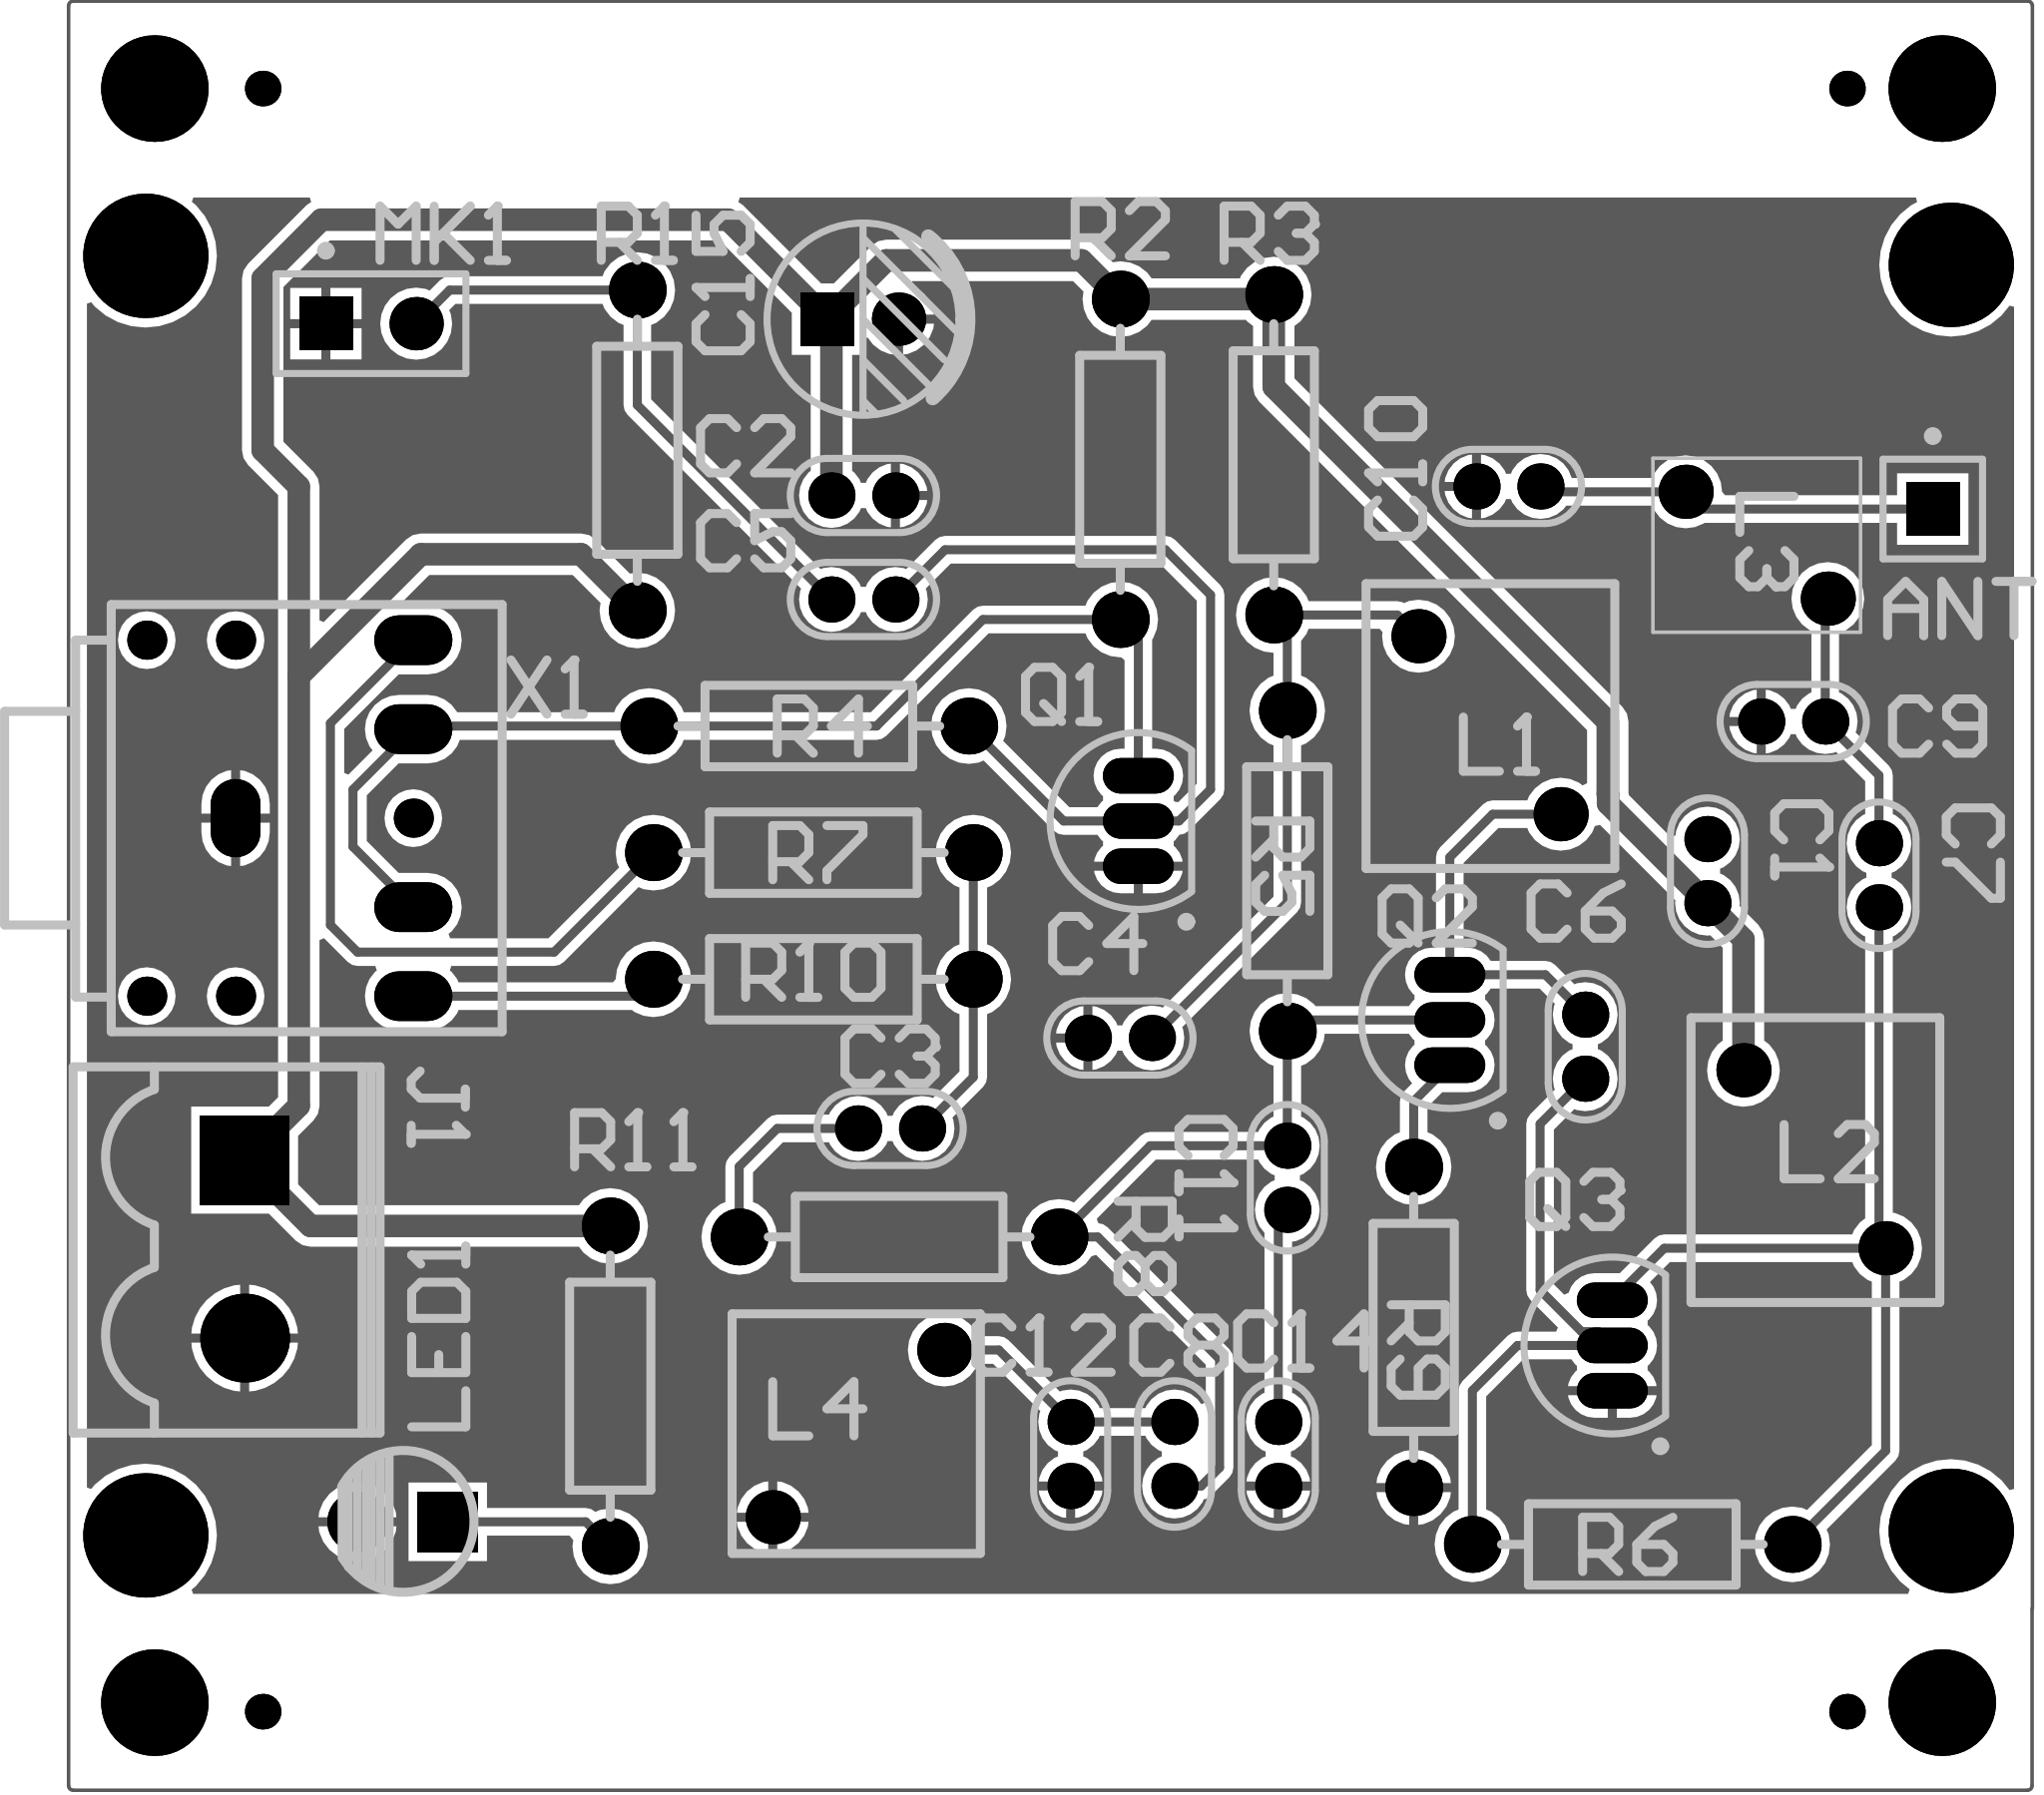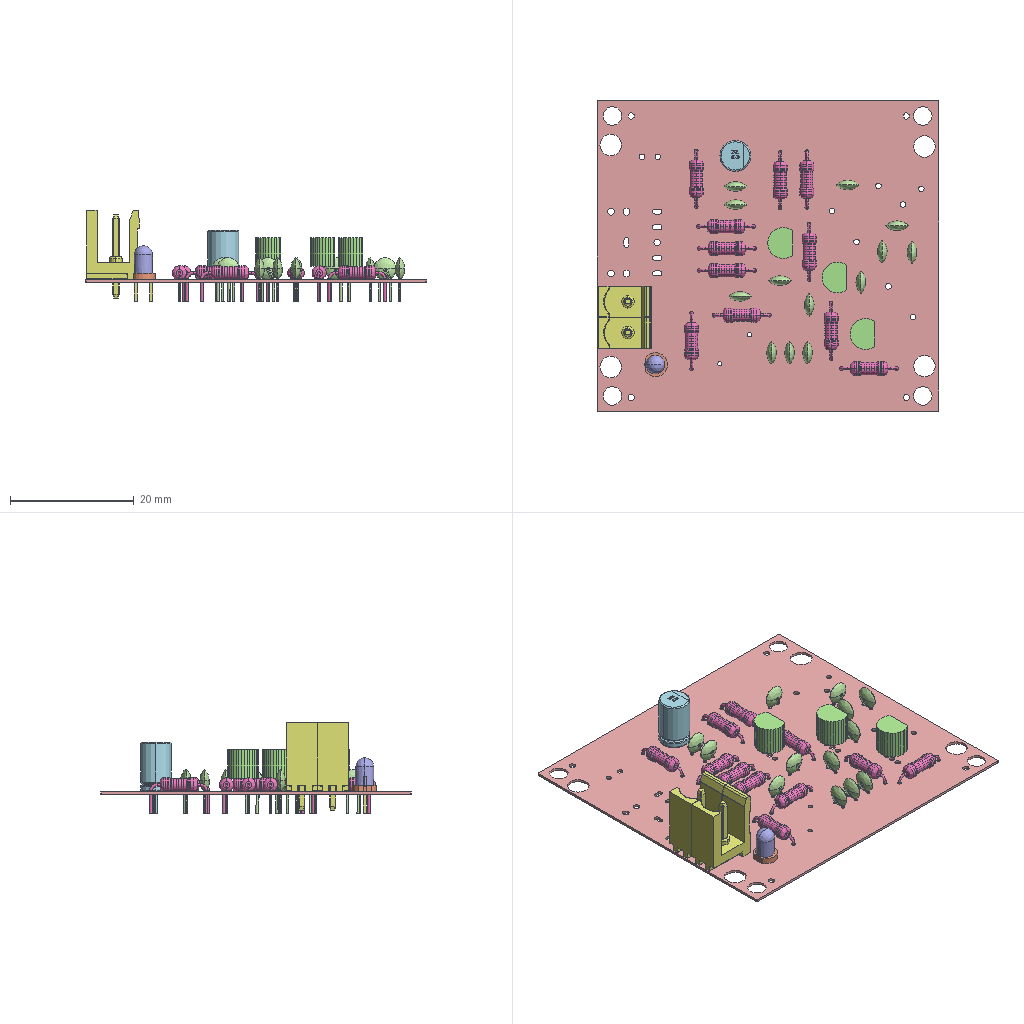Circuit board layout | Altium Designer | box 55.3 x 50.3 x 14.8 mm
Layer stack:
# Altium Designer layer stack of  (unit mm; dielectric type: 0 none, 1 core, 2 prepreg, 3 surface material)
index,name,kind,layer,copper_thickness_mm,dielectric_type,dielectric_thickness_mm,dielectric_material,dielectric_constant
0,Top Paste,other,,,,,,
1,Top Overlay,other,,,,,,
2,Top Solder,dielectric,,,3,0.0102,Solder Resist,3.5
3,Top Layer,copper,Top Layer,0.0356,,,,
4,Dielectric 1,dielectric,,,0,0.32,FR-4,4.8
5,Bottom Layer,copper,Bottom Layer,0.0356,,,,
6,Bottom Solder,dielectric,,,3,0.0102,Solder Resist,3.5
7,Bottom Overlay,other,,,,,,
8,Bottom Paste,other,,,,,,
# drill layer pairs: low layer,high layer
drill_pair,Top Layer,Bottom Layer
Part placement:
Designator,Comment,Layer,Footprint,Center-X(mm),Center-Y(mm),Rotation
ANT,Antenna,TopLayer,PIN1,77.724,56.261,0
C1,102,TopLayer,CC_1.8*3.6,71.385,46.09,270
C2,104,TopLayer,CC_1.8*3.6,47.636,56.642,180
C3,104,TopLayer,CC_1.8*3.6,48.387,38.862,180
C4,102,TopLayer,CC_1.8*3.6,54.853,41.402,0
C5,104,TopLayer,CC_1.8*3.6,47.636,53.721,0
C6,101,TopLayer,CC_1.8*3.6,67.945,41.159,90
C7,30P,TopLayer,CC_1.8*3.6,76.211,45.974,270
C8,30P,TopLayer,CC_1.8*3.6,56.388,29.718,90
C9,101,TopLayer,CC_1.8*3.6,73.798,50.292,180
C10,30,TopLayer,CC_1.8*3.6,65.786,56.896,180
C11,68P,TopLayer,CC_1.8*3.6,59.563,37.476,270
C12,15P,TopLayer,CC_1.8*3.6,53.467,29.718,270
C14,101,TopLayer,CC_1.8*3.6,59.309,29.718,270
C15,47UF,TopLayer,CS_2.0*5*8_-_C,47.625,61.595,180
L1,Air-core inductor 8T,TopLayer,8T,65.254,50.189,180
L2,Air-core inductor 8T,TopLayer,8T,74.398,37.997,180
L3,Air-core inductor 5T,TopLayer,5T,72.771,55.245,270
L4,Adjustable inductor 7T,TopLayer,可调电感7T,47.498,30.289,0
LED1,Red,TopLayer,LED_3MM-B,34.671,27.813,180
MK1,Mic2,TopLayer,PIN2,33.782,61.468,0
Q1,9014,TopLayer,TO-92A,55.372,47.498,0
Q2,9018,TopLayer,TO-92A,64.135,41.91,0
Q3,9018,TopLayer,TO-92A,68.707,32.766,0
R1,10K,TopLayer,RS_1/4W,41.275,57.912,270
R2,10K,TopLayer,RS_1/4W,54.864,57.658,90
R3,100,TopLayer,RS_1/4W,59.182,57.785,270
R4,100K,TopLayer,RS_1/4W,46.101,50.165,360
R5,47K,TopLayer,RS_1/4W,59.563,46.101,270
R6,47K,TopLayer,RS_1/4W,69.27,27.178,180
R7,10K,TopLayer,RS_1/4W,46.228,46.609,360
R8,22K,TopLayer,RS_1/4W,48.641,35.814,360
R9,470,TopLayer,RS_1/4W,63.119,33.274,270
R10,10K,TopLayer,RS_1/4W,46.228,43.053,360
R11,10K,TopLayer,RS_1/4W,40.513,31.623,90
X1,3F07,TopLayer,3F07,31.222,47.578,0
J1,KF2EDGK-2P,TopLayer,KF2EDGK5.0-2P,30.226,35.473,270
Pad and via stacks:
# Altium Designer via and pad stacks of  (unit mm). Each distinct definition once, with the count of objects using it.
# via: kind,start_layer,end_layer,hole_mm,diameter_mm,mode(0 simple;1 top-mid-bottom;2 full stack),diameter_per_layer,count,example_net
# pad: kind,layer,hole_mm,hole_type(0 round;1 square;2 slot),plating,top_size,top_shape(1 round;2 rect;3 octagon;9 rounded rect),mid_size,bottom_size,mode,footprint,size_per_layer,count,example
pad,Multi-Layer,0.5,0,plated,1.3x1.3,1,1.3x1.3,1.3x1.3,0,CC 1.8*3.6,,26,C14.1
pad,Multi-Layer,0.6,0,plated,1.6x1.6,1,1.6x1.6,1.6x1.6,0,RS 1/4W,,22,R9.1
pad,Multi-Layer,0.7,0,plated,1.524x1.524,1,1.524x1.524,1.524x1.524,0,\u00BF\u00C9\u00B5\u00F7\u00B5\u00E7\u00B8\u00D07T,,2,L4.2
pad,Multi-Layer,0.9,0,plated,2x1,1,2x1,2x1,0,TO-92A,,9,Q2.1
pad,Multi-Layer,1.1,0,unplated,1.1x1.1,1,1.1x1.1,1.1x1.1,0,3F07,,5,X1.
pad,Multi-Layer,0.8,2,plated,2.2x1.4,1,2.2x1.4,2.2x1.4,0,3F07,,5,X1.1
pad,Multi-Layer,0.9144,0,plated,1.524x1.524,1,1.524x1.524,1.524x1.524,0,8T,,4,L1.2
pad,Multi-Layer,0.9144,0,plated,1.524x1.524,1,1.524x1.524,1.524x1.524,0,5T,,2,L3.1
pad,Multi-Layer,0.9,0,plated,1.5x1.5,1,1.5x1.5,1.5x1.5,0,PIN2,,1,MK1.2
pad,Multi-Layer,0.9,0,plated,1.5x1.5,2,1.5x1.5,1.5x1.5,0,PIN2,,1,MK1.1
pad,Multi-Layer,0.9,0,plated,1.7x1.7,1,1.7x1.7,1.7x1.7,0,LED 3MM-B,,1,LED1.2
pad,Multi-Layer,0.9,0,plated,1.7x1.7,2,1.7x1.7,1.7x1.7,0,LED 3MM-B,,1,LED1.1
pad,Multi-Layer,0.9,0,plated,1.5x1.5,2,1.5x1.5,1.5x1.5,0,PIN1,,1,ANT.1
pad,Multi-Layer,0.8,0,plated,1.5x1.5,1,1.5x1.5,1.5x1.5,0,CS 2.0*5*8 - C,,1,C15.2
pad,Multi-Layer,0.8,0,plated,1.5x1.5,2,1.5x1.5,1.5x1.5,0,CS 2.0*5*8 - C,,1,C15.1
pad,Multi-Layer,1.6,0,plated,2.5x2.5,2,2.5x2.5,2.5x2.5,0,KF2EDGK5.0-2P,,1,J1.1
pad,Multi-Layer,1.6,0,plated,2.5x2.5,1,2.5x2.5,2.5x2.5,0,KF2EDGK5.0-2P,,1,J1.2
pad,Multi-Layer,3.5,0,plated,3.5x3.5,1,3.5x3.5,3.5x3.5,0,,,4,0
pad,Multi-Layer,3,0,plated,3x3,1,3x3,3x3,0,,,4,4
pad,Multi-Layer,1,0,plated,1x1,1,1x1,1x1,0,,,4,6
Copper pours:
name,layer,net,type(0 solid;1 hatched;2 none)
G,Bottom Layer,GND,0
Design rules, without the lines most boards share:
# Altium Designer design rules of  (exported by Altium Designer, unit mm)
# columns: name | kind | enabled | priority | scope1 | scope2 | descriptor | typed fields (field=value)
NetAntennae | 56 | enabled | 1 | All | All | Net Antennae (Tolerance=0mm) (All) |
SilkToSilkClearance | 55 | enabled | 1 | All | All | Silk to Silk (Clearance=0mm) (All),(All) |
SilkToSolderMaskClearance | 54 | enabled | 1 | IsPad | All | Silk To Solder Mask (Clearance=0mm) (IsPad),(All) |
MinimumSolderMaskSliver | 53 | enabled | 1 | All | All | Minimum Solder Mask Sliver (Gap=0mm) (All),(All) |
HoleToHoleClearance | 52 | enabled | 1 | All | All | Hole To Hole Clearance (Gap=0.254mm) (All),(All) | gap=0.254
DiffPairsRouting | 51 | enabled | 1 | All | All | Differential Pairs Uncoupled Length using the Gap Constraints (Min=0.254mm) (Max=0.254mm) (Prefered=0.254mm)  and Width Constraints (Min=0.381mm) (Max=0.381mm) (Prefered=0.381mm) (All) |
HoleSize | 42 | enabled | 1 | All | All | Hole Size Constraint (Min=0.025mm) (Max=2.54mm) (All) |
Height | 50 | enabled | 1 | All | All | Height Constraint (Min=0mm) (Max=25.4mm) (Prefered=12.7mm) (All) | min_height=0 max_height=25.4
ComponentClearance | 24 | enabled | 1 | All | All | Component Clearance Constraint ( Horizontal Gap = 0.254mm, Vertical Gap = 0.254mm ) (All),(All)  | gap=0.254
SolderMaskExpansion | 13 | enabled | 1 | All | All | Solder Mask Expansion (Expansion =0.102mm) (All) | expansion=0.1016
PasteMaskExpansion | 14 | enabled | 1 | All | All | Paste Mask Expansion (Expansion =0mm) (All) | expansion=0
RoutingVias | 11 | enabled | 1 | All | All | Routing Via (MinHoleWidth=0.711mm) (MaxHoleWidth=0.711mm) (PreferredHoleWidth=0.711mm) (MinWidth=1.27mm) (MaxWidth=1.27mm) (PreferedWidth=1.27mm) (All) | via_min_hole=0.7112 via_max_hole=0.7112 via_preferred_diameter=1.27 via_preferred_hole=0.7112
RoutingCorners | 10 | enabled | 1 | All | All | Routing Corners (Style=45-Degree) (Min Setback=2.54mm) (Max Setback=2.54mm) (All) |
Width | 2 | enabled | 1 | All | All | Width Constraint (Min=0.254mm) (Max=20mm) (Preferred=0.254mm) (All) |
PolygonConnect | 20 | enabled | 1 | All | All | Polygon Connect Rule(Relief Connect )(Conductor Width=0.254mm) (Relief Angle=90 Angle) (Entries=4) (Air Gap Width=0.254mm) (All),(All) | connect_style(0=relief,1=direct,2=none)=0 relief_conductor_width=0.254 relief_entries=4
PlaneClearance | 12 | enabled | 1 | All | All | Power Plane Clearance (Clearance =0.508mm) (All) | clearance=0.508
PlaneConnect | 6 | enabled | 1 | All | All | Power Plane Connect Rule(Relief Connect )(Expansion=0.508mm) (Conductor Width=0.254mm) (Air Gap=0.254mm) (Entries=4) (All) | relief_conductor_width=0.254 relief_entries=4 relief_expansion=0.508
Clearance | 0 | enabled | 1 | All | All | Clearance Constraint (Gap=0.254mm) (All),(All) | gap=0.254
Classes set for this board:
# Altium Designer classes of  (member kind: 0 net, 1 component, 2 from-to, 3 pad, 4 layer, 5 differential pair, 6 design channel, 7 polygon, 8 structure, 9 xSignal)
# columns: class name | member kind | superclass | members
Sheet1 | 1 | no | ANT; C1; C2; C3; C4; C5; C6; C7; C8; C9; C10; C11; C12; C14; C15; L1; L2; L3; L4; LED1; MK1; Q1; Q2; Q3; R1; R2; R3; R4; R5; R6; R7; R8; R9; R10; R11; X1;